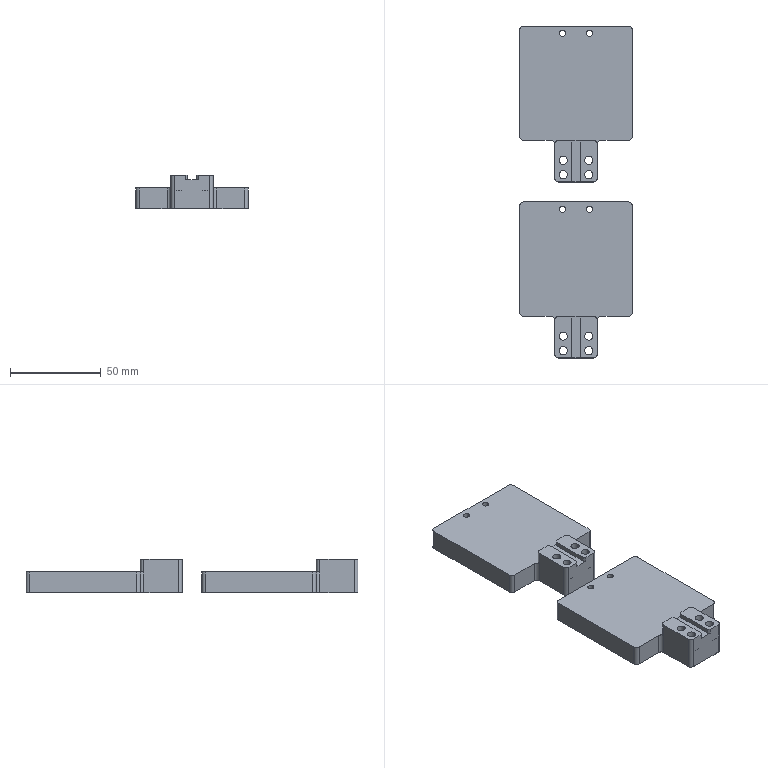NC program | NX | posted with a generic post | part box 62 x 183 x 18.5 mm
Whole program:
N10 G17 G21 G94 G90
(FLOOR_WALL_COPY , TOOL : D80)
N12 T19 M6
N14 G54
N16 G17 G0 G90 X226. Y31. S6500 M3
N18 G43 Z30. H19
N20 Z9.
N22 G94 G1 Z6. F1500.
N24 X223.
N26 X-40.
N28 X-43.
N30 Z9.
N32 G0 Z30.
N34 X226.
N36 Z8.
N38 G1 Z5.
N40 X223.
N42 X-40.
N44 X-43.
N46 Z8.
N48 G0 Z30.
N50 X226.
N52 Z7.
N54 G1 Z4.
N56 X223.
N58 X-40.
N60 X-43.
N62 Z7.
N64 G0 Z30.
N66 X226.
N68 Z6.
N70 G1 Z3.
N72 X223.
N74 X-40.
N76 X-43.
N78 Z6.
N80 G0 Z30.
N82 X226.
N84 Z5.
N86 G1 Z2.
N88 X223.
N90 X-40.
N92 X-43.
N94 Z5.
N96 G0 Z30.
N98 X226.
N100 Z4.
N102 G1 Z1.
N104 X223.
N106 X-40.
N108 X-43.
N110 Z4.
N112 G0 Z30.
N114 X226.
N116 Z3.
N118 G1 Z0.
N120 X223.
N122 X-40.
N124 X-43.
N126 Z3.
N128 G0 Z30.
N130 M5
(FLOOR_WALL_1 , TOOL : D10)
N132 T15 M6
N134 G54
N136 G17 G0 G90 X-6.5 Y26.67 S9500 M3
N138 G43 Z30. H15
N140 Z0.514
N142 G94 G1 Z-0.986 F1000.
N144 X-0.5 Y30.134
N146 G3 X0. Y31. R1.
N148 G1 Y60. F3500.
N150 G2 X2. Y62. R2.
N152 G1 X61.
N154 G2 X63. Y60. R2.
N156 G1 Y47.512
N158 G3 X57.9 Y40.7 R7.1
N160 G1 Y21.3
N162 G3 X63. Y14.488 R7.1
N164 G1 Y2.
N166 G2 X61. Y0. R2.
N168 G1 X2.
N170 G2 X0. Y2. R2.
N172 G1 Y31.
N174 X5.
N176 Y57.
N178 X58.
N180 Y50.57
N182 G3 X52.9 Y40.7 R12.1
N184 G1 Y21.3
N186 G3 X58. Y11.43 R12.1
N188 G1 Y5.
N190 X5.
N192 Y31.
N194 X10.
N196 Y52.
N198 X52.166
N200 G3 X47.9 Y40.7 R17.1
N202 G1 Y21.3
N204 G3 X52.166 Y10. R17.1
N206 G1 X10.
N208 Y31.
N210 X15.
N212 Y47.
N214 X43.817
N216 G3 X42.9 Y40.7 R22.1
N218 G1 Y21.3
N220 G3 X43.817 Y15. R22.1
N222 G1 X15.
N224 Y31.
N226 X20.
N228 Y42.
N230 X37.931
N232 G3 X37.9 Y40.7 R27.1
N234 G1 Y21.3
N236 G3 X37.931 Y20. R27.1
N238 G1 X20.
N240 Y31.
N242 X25.
N244 Y37.
N246 X32.9
N248 Y25.
N250 X25.
N252 Y31.
N254 G3 X24.5 Y31.866 R1.
N256 G1 Z0.514
N258 G0 X-6.5 Y26.67 Z-0.471
N260 G1 Z-1.971 F1000.
N262 X-0.5 Y30.134
N264 G3 X0. Y31. R1.
N266 G1 Y60. F3500.
N268 G2 X2. Y62. R2.
N270 G1 X61.
N272 G2 X63. Y60. R2.
N274 G1 Y47.512
N276 G3 X57.9 Y40.7 R7.1
N278 G1 Y21.3
N280 G3 X63. Y14.488 R7.1
N282 G1 Y2.
N284 G2 X61. Y0. R2.
N286 G1 X2.
N288 G2 X0. Y2. R2.
N290 G1 Y31.
N292 X5.
N294 Y57.
N296 X58.
N298 Y50.57
N300 G3 X52.9 Y40.7 R12.1
N302 G1 Y21.3
N304 G3 X58. Y11.43 R12.1
N306 G1 Y5.
N308 X5.
N310 Y31.
N312 X10.
N314 Y52.
N316 X52.166
N318 G3 X47.9 Y40.7 R17.1
N320 G1 Y21.3
N322 G3 X52.166 Y10. R17.1
N324 G1 X10.
N326 Y31.
N328 X15.
N330 Y47.
N332 X43.817
N334 G3 X42.9 Y40.7 R22.1
N336 G1 Y21.3
N338 G3 X43.817 Y15. R22.1
N340 G1 X15.
N342 Y31.
N344 X20.
N346 Y42.
N348 X37.931
N350 G3 X37.9 Y40.7 R27.1
N352 G1 Y21.3
N354 G3 X37.931 Y20. R27.1
N356 G1 X20.
N358 Y31.
N360 X25.
N362 Y37.
N364 X32.9
N366 Y25.
N368 X25.
N370 Y31.
N372 G3 X24.5 Y31.866 R1.
N374 G1 Z-0.471
N376 G0 X-6.5 Y26.67 Z-1.457
N378 G1 Z-2.957 F1000.
N380 X-0.5 Y30.134
N382 G3 X0. Y31. R1.
N384 G1 Y60. F3500.
N386 G2 X2. Y62. R2.
N388 G1 X61.
N390 G2 X63. Y60. R2.
N392 G1 Y47.512
N394 G3 X57.9 Y40.7 R7.1
N396 G1 Y21.3
N398 G3 X63. Y14.488 R7.1
N400 G1 Y2.
N402 G2 X61. Y0. R2.
N404 G1 X2.
N406 G2 X0. Y2. R2.
N408 G1 Y31.
N410 X5.
N412 Y57.
N414 X58.
N416 Y50.57
N418 G3 X52.9 Y40.7 R12.1
N420 G1 Y21.3
N422 G3 X58. Y11.43 R12.1
N424 G1 Y5.
N426 X5.
N428 Y31.
N430 X10.
N432 Y52.
N434 X52.166
N436 G3 X47.9 Y40.7 R17.1
N438 G1 Y21.3
N440 G3 X52.166 Y10. R17.1
N442 G1 X10.
N444 Y31.
N446 X15.
N448 Y47.
N450 X43.817
N452 G3 X42.9 Y40.7 R22.1
N454 G1 Y21.3
N456 G3 X43.817 Y15. R22.1
N458 G1 X15.
N460 Y31.
N462 X20.
N464 Y42.
N466 X37.931
N468 G3 X37.9 Y40.7 R27.1
N470 G1 Y21.3
N472 G3 X37.931 Y20. R27.1
N474 G1 X20.
N476 Y31.
N478 X25.
N480 Y37.
N482 X32.9
N484 Y25.
N486 X25.
N488 Y31.
N490 G3 X24.5 Y31.866 R1.
N492 G1 Z-1.457
N494 G0 X-6.5 Y26.67 Z-2.443
N496 G1 Z-3.943 F1000.
N498 X-0.5 Y30.134
N500 G3 X0. Y31. R1.
N502 G1 Y60. F3500.
N504 G2 X2. Y62. R2.
N506 G1 X61.
N508 G2 X63. Y60. R2.
N510 G1 Y47.512
N512 G3 X57.9 Y40.7 R7.1
N514 G1 Y21.3
N516 G3 X63. Y14.488 R7.1
N518 G1 Y2.
N520 G2 X61. Y0. R2.
N522 G1 X2.
N524 G2 X0. Y2. R2.
N526 G1 Y31.
N528 X5.
N530 Y57.
N532 X58.
N534 Y50.57
N536 G3 X52.9 Y40.7 R12.1
N538 G1 Y21.3
N540 G3 X58. Y11.43 R12.1
N542 G1 Y5.
N544 X5.
N546 Y31.
N548 X10.
N550 Y52.
N552 X52.166
N554 G3 X47.9 Y40.7 R17.1
N556 G1 Y21.3
N558 G3 X52.166 Y10. R17.1
N560 G1 X10.
N562 Y31.
N564 X15.
N566 Y47.
N568 X43.817
N570 G3 X42.9 Y40.7 R22.1
N572 G1 Y21.3
N574 G3 X43.817 Y15. R22.1
N576 G1 X15.
N578 Y31.
N580 X20.
N582 Y42.
N584 X37.931
N586 G3 X37.9 Y40.7 R27.1
N588 G1 Y21.3
N590 G3 X37.931 Y20. R27.1
N592 G1 X20.
N594 Y31.
N596 X25.
N598 Y37.
N600 X32.9
N602 Y25.
N604 X25.
N606 Y31.
N608 G3 X24.5 Y31.866 R1.
N610 G1 Z-2.443
N612 G0 X-6.5 Y26.67 Z-3.429
N614 G1 Z-4.929 F1000.
N616 X-0.5 Y30.134
N618 G3 X0. Y31. R1.
N620 G1 Y60. F3500.
N622 G2 X2. Y62. R2.
N624 G1 X61.
N626 G2 X63. Y60. R2.
N628 G1 Y47.512
N630 G3 X57.9 Y40.7 R7.1
N632 G1 Y21.3
N634 G3 X63. Y14.488 R7.1
N636 G1 Y2.
N638 G2 X61. Y0. R2.
N640 G1 X2.
N642 G2 X0. Y2. R2.
N644 G1 Y31.
N646 X5.
N648 Y57.
N650 X58.
N652 Y50.57
N654 G3 X52.9 Y40.7 R12.1
N656 G1 Y21.3
N658 G3 X58. Y11.43 R12.1
N660 G1 Y5.
N662 X5.
N664 Y31.
N666 X10.
N668 Y52.
N670 X52.166
N672 G3 X47.9 Y40.7 R17.1
N674 G1 Y21.3
N676 G3 X52.166 Y10. R17.1
N678 G1 X10.
N680 Y31.
N682 X15.
N684 Y47.
N686 X43.817
N688 G3 X42.9 Y40.7 R22.1
N690 G1 Y21.3
N692 G3 X43.817 Y15. R22.1
N694 G1 X15.
N696 Y31.
N698 X20.
N700 Y42.
N702 X37.931
N704 G3 X37.9 Y40.7 R27.1
N706 G1 Y21.3
N708 G3 X37.931 Y20. R27.1
N710 G1 X20.
N712 Y31.
N714 X25.
N716 Y37.
N718 X32.9
N720 Y25.
N722 X25.
N724 Y31.
N726 G3 X24.5 Y31.866 R1.
N728 G1 Z-3.429
N730 G0 X-6.5 Y26.67 Z-4.414
N732 G1 Z-5.914 F1000.
N734 X-0.5 Y30.134
N736 G3 X0. Y31. R1.
N738 G1 Y60. F3500.
N740 G2 X2. Y62. R2.
N742 G1 X61.
N744 G2 X63. Y60. R2.
N746 G1 Y47.512
N748 G3 X57.9 Y40.7 R7.1
N750 G1 Y21.3
N752 G3 X63. Y14.488 R7.1
N754 G1 Y2.
N756 G2 X61. Y0. R2.
N758 G1 X2.
N760 G2 X0. Y2. R2.
N762 G1 Y31.
N764 X5.
N766 Y57.
N768 X58.
N770 Y50.57
N772 G3 X52.9 Y40.7 R12.1
N774 G1 Y21.3
N776 G3 X58. Y11.43 R12.1
N778 G1 Y5.
N780 X5.
N782 Y31.
N784 X10.
N786 Y52.
N788 X52.166
N790 G3 X47.9 Y40.7 R17.1
N792 G1 Y21.3
N794 G3 X52.166 Y10. R17.1
N796 G1 X10.
N798 Y31.
N800 X15.
N802 Y47.
N804 X43.817
N806 G3 X42.9 Y40.7 R22.1
N808 G1 Y21.3
N810 G3 X43.817 Y15. R22.1
N812 G1 X15.
N814 Y31.
N816 X20.
N818 Y42.
N820 X37.931
N822 G3 X37.9 Y40.7 R27.1
N824 G1 Y21.3
N826 G3 X37.931 Y20. R27.1
N828 G1 X20.
N830 Y31.
N832 X25.
N834 Y37.
N836 X32.9
N838 Y25.
N840 X25.
N842 Y31.
N844 G3 X24.5 Y31.866 R1.
N846 G1 Z-4.414
N848 G0 X-6.5 Y26.67 Z-5.4
N850 G1 Z-6.9 F1000.
N852 X-0.5 Y30.134
N854 G3 X0. Y31. R1.
N856 G1 Y60. F3500.
N858 G2 X2. Y62. R2.
N860 G1 X61.
N862 G2 X63. Y60. R2.
N864 G1 Y47.512
N866 G3 X57.9 Y40.7 R7.1
N868 G1 Y21.3
N870 G3 X63. Y14.488 R7.1
N872 G1 Y2.
N874 G2 X61. Y0. R2.
N876 G1 X2.
N878 G2 X0. Y2. R2.
N880 G1 Y31.
N882 X5.
N884 Y57.
N886 X58.
N888 Y50.57
N890 G3 X52.9 Y40.7 R12.1
N892 G1 Y21.3
N894 G3 X58. Y11.43 R12.1
N896 G1 Y5.
N898 X5.
N900 Y31.
N902 X10.
N904 Y52.
N906 X52.166
N908 G3 X47.9 Y40.7 R17.1
N910 G1 Y21.3
N912 G3 X52.166 Y10. R17.1
N914 G1 X10.
N916 Y31.
N918 X15.
N920 Y47.
N922 X43.817
N924 G3 X42.9 Y40.7 R22.1
N926 G1 Y21.3
N928 G3 X43.817 Y15. R22.1
N930 G1 X15.
N932 Y31.
N934 X20.
N936 Y42.
N938 X37.931
N940 G3 X37.9 Y40.7 R27.1
N942 G1 Y21.3
N944 G3 X37.931 Y20. R27.1
N946 G1 X20.
N948 Y31.
N950 X25.
N952 Y37.
N954 X32.9
N956 Y25.
N958 X25.
N960 Y31.
N962 G3 X24.5 Y31.866 R1.
N964 G1 Z-5.4
N966 G0 Z30.
N968 X130.28 Y-6.5
N970 Z0.514
N972 G1 Z-0.986 F1000.
N974 X126.816 Y-0.5
N976 G3 X125.95 Y0. R1.
N978 G1 X99. F3500.
N980 G2 X97. Y2. R2.
N982 G1 Y60.
N984 G2 X99. Y62. R2.
N986 G1 X158.
N988 G2 X160. Y60. R2.
N990 G1 Y47.512
N992 G3 X154.9 Y40.7 R7.1
N994 G1 Y21.3
N996 G3 X160. Y14.488 R7.1
N998 G1 Y2.
N1000 G2 X158. Y0. R2.
N1002 G1 X125.95
N1004 Y5.
N1006 X102.
N1008 Y57.
N1010 X155.
N1012 Y50.57
N1014 G3 X149.9 Y40.7 R12.1
N1016 G1 Y21.3
N1018 G3 X155. Y11.43 R12.1
N1020 G1 Y5.
N1022 X125.95
N1024 Y10.
N1026 X107.
N1028 Y52.
N1030 X149.166
N1032 G3 X144.9 Y40.7 R17.1
N1034 G1 Y21.3
N1036 G3 X149.166 Y10. R17.1
N1038 G1 X125.95
N1040 Y15.
N1042 X112.
N1044 Y47.
N1046 X140.817
N1048 G3 X139.9 Y40.7 R22.1
N1050 G1 Y21.3
N1052 G3 X140.817 Y15. R22.1
N1054 G1 X125.95
N1056 Y20.
N1058 X117.
N1060 Y42.
N1062 X134.931
N1064 G3 X134.9 Y40.7 R27.1
N1066 G1 Y21.3
N1068 G3 X134.931 Y20. R27.1
N1070 G1 X125.95
N1072 Y25.
N1074 X122.
N1076 Y37.
N1078 X129.9
N1080 Y25.
N1082 X125.95
N1084 G3 X125.084 Y24.5 R1.
N1086 G1 Z0.514
N1088 G0 X130.28 Y-6.5 Z-0.471
N1090 G1 Z-1.971 F1000.
N1092 X126.816 Y-0.5
N1094 G3 X125.95 Y0. R1.
N1096 G1 X99. F3500.
N1098 G2 X97. Y2. R2.
N1100 G1 Y60.
N1102 G2 X99. Y62. R2.
N1104 G1 X158.
N1106 G2 X160. Y60. R2.
N1108 G1 Y47.512
N1110 G3 X154.9 Y40.7 R7.1
N1112 G1 Y21.3
N1114 G3 X160. Y14.488 R7.1
N1116 G1 Y2.
N1118 G2 X158. Y0. R2.
N1120 G1 X125.95
N1122 Y5.
N1124 X102.
N1126 Y57.
N1128 X155.
N1130 Y50.57
N1132 G3 X149.9 Y40.7 R12.1
N1134 G1 Y21.3
N1136 G3 X155. Y11.43 R12.1
N1138 G1 Y5.
N1140 X125.95
N1142 Y10.
N1144 X107.
N1146 Y52.
N1148 X149.166
N1150 G3 X144.9 Y40.7 R17.1
N1152 G1 Y21.3
N1154 G3 X149.166 Y10. R17.1
N1156 G1 X125.95
N1158 Y15.
N1160 X112.
N1162 Y47.
N1164 X140.817
N1166 G3 X139.9 Y40.7 R22.1
N1168 G1 Y21.3
N1170 G3 X140.817 Y15. R22.1
N1172 G1 X125.95
N1174 Y20.
N1176 X117.
N1178 Y42.
N1180 X134.931
N1182 G3 X134.9 Y40.7 R27.1
N1184 G1 Y21.3
N1186 G3 X134.931 Y20. R27.1
N1188 G1 X125.95
N1190 Y25.
N1192 X122.
N1194 Y37.
N1196 X129.9
N1198 Y25.
N1200 X125.95
N1202 G3 X125.084 Y24.5 R1.
N1204 G1 Z-0.471
N1206 G0 X130.28 Y-6.5 Z-1.457
N1208 G1 Z-2.957 F1000.
N1210 X126.816 Y-0.5
N1212 G3 X125.95 Y0. R1.
N1214 G1 X99. F3500.
N1216 G2 X97. Y2. R2.
N1218 G1 Y60.
N1220 G2 X99. Y62. R2.
N1222 G1 X158.
N1224 G2 X160. Y60. R2.
N1226 G1 Y47.512
N1228 G3 X154.9 Y40.7 R7.1
N1230 G1 Y21.3
N1232 G3 X160. Y14.488 R7.1
N1234 G1 Y2.
N1236 G2 X158. Y0. R2.
N1238 G1 X125.95
N1240 Y5.
N1242 X102.
N1244 Y57.
N1246 X155.
N1248 Y50.57
N1250 G3 X149.9 Y40.7 R12.1
N1252 G1 Y21.3
N1254 G3 X155. Y11.43 R12.1
N1256 G1 Y5.
N1258 X125.95
N1260 Y10.
N1262 X107.
N1264 Y52.
N1266 X149.166
N1268 G3 X144.9 Y40.7 R17.1
N1270 G1 Y21.3
N1272 G3 X149.166 Y10. R17.1
N1274 G1 X125.95
N1276 Y15.
N1278 X112.
N1280 Y47.
N1282 X140.817
N1284 G3 X139.9 Y40.7 R22.1
N1286 G1 Y21.3
N1288 G3 X140.817 Y15. R22.1
N1290 G1 X125.95
N1292 Y20.
N1294 X117.
N1296 Y42.
N1298 X134.931
N1300 G3 X134.9 Y40.7 R27.1
N1302 G1 Y21.3
N1304 G3 X134.931 Y20. R27.1
N1306 G1 X125.95
N1308 Y25.
N1310 X122.
N1312 Y37.
N1314 X129.9
N1316 Y25.
N1318 X125.95
N1320 G3 X125.084 Y24.5 R1.
N1322 G1 Z-1.457
N1324 G0 X130.28 Y-6.5 Z-2.443
N1326 G1 Z-3.943 F1000.
N1328 X126.816 Y-0.5
N1330 G3 X125.95 Y0. R1.
N1332 G1 X99. F3500.
N1334 G2 X97. Y2. R2.
N1336 G1 Y60.
N1338 G2 X99. Y62. R2.
N1340 G1 X158.
N1342 G2 X160. Y60. R2.
N1344 G1 Y47.512
N1346 G3 X154.9 Y40.7 R7.1
N1348 G1 Y21.3
N1350 G3 X160. Y14.488 R7.1
N1352 G1 Y2.
N1354 G2 X158. Y0. R2.
N1356 G1 X125.95
N1358 Y5.
N1360 X102.
N1362 Y57.
N1364 X155.
N1366 Y50.57
N1368 G3 X149.9 Y40.7 R12.1
N1370 G1 Y21.3
N1372 G3 X155. Y11.43 R12.1
N1374 G1 Y5.
N1376 X125.95
N1378 Y10.
N1380 X107.
N1382 Y52.
N1384 X149.166
N1386 G3 X144.9 Y40.7 R17.1
N1388 G1 Y21.3
N1390 G3 X149.166 Y10. R17.1
N1392 G1 X125.95
N1394 Y15.
N1396 X112.
N1398 Y47.
N1400 X140.817
N1402 G3 X139.9 Y40.7 R22.1
N1404 G1 Y21.3
N1406 G3 X140.817 Y15. R22.1
N1408 G1 X125.95
N1410 Y20.
N1412 X117.
N1414 Y42.
N1416 X134.931
N1418 G3 X134.9 Y40.7 R27.1
N1420 G1 Y21.3
N1422 G3 X134.931 Y20. R27.1
N1424 G1 X125.95
N1426 Y25.
N1428 X122.
N1430 Y37.
N1432 X129.9
N1434 Y25.
N1436 X125.95
N1438 G3 X125.084 Y24.5 R1.
N1440 G1 Z-2.443
N1442 G0 X130.28 Y-6.5 Z-3.429
N1444 G1 Z-4.929 F1000.
N1446 X126.816 Y-0.5
N1448 G3 X125.95 Y0. R1.
N1450 G1 X99. F3500.
N1452 G2 X97. Y2. R2.
N1454 G1 Y60.
N1456 G2 X99. Y62. R2.
N1458 G1 X158.
N1460 G2 X160. Y60. R2.
N1462 G1 Y47.512
N1464 G3 X154.9 Y40.7 R7.1
N1466 G1 Y21.3
N1468 G3 X160. Y14.488 R7.1
N1470 G1 Y2.
N1472 G2 X158. Y0. R2.
N1474 G1 X125.95
N1476 Y5.
N1478 X102.
N1480 Y57.
N1482 X155.
N1484 Y50.57
N1486 G3 X149.9 Y40.7 R12.1
N1488 G1 Y21.3
N1490 G3 X155. Y11.43 R12.1
N1492 G1 Y5.
N1494 X125.95
N1496 Y10.
N1498 X107.
N1500 Y52.
N1502 X149.166
N1504 G3 X144.9 Y40.7 R17.1
N1506 G1 Y21.3
N1508 G3 X149.166 Y10. R17.1
N1510 G1 X125.95
N1512 Y15.
N1514 X112.
N1516 Y47.
N1518 X140.817
N1520 G3 X139.9 Y40.7 R22.1
N1522 G1 Y21.3
N1524 G3 X140.817 Y15. R22.1
N1526 G1 X125.95
N1528 Y20.
N1530 X117.
N1532 Y42.
N1534 X134.931
N1536 G3 X134.9 Y40.7 R27.1
N1538 G1 Y21.3
N1540 G3 X134.931 Y20. R27.1
N1542 G1 X125.95
N1544 Y25.
N1546 X122.
N1548 Y37.
N1550 X129.9
N1552 Y25.
N1554 X125.95
N1556 G3 X125.084 Y24.5 R1.
N1558 G1 Z-3.429
N1560 G0 X130.28 Y-6.5 Z-4.414
N1562 G1 Z-5.914 F1000.
N1564 X126.816 Y-0.5
N1566 G3 X125.95 Y0. R1.
N1568 G1 X99. F3500.
N1570 G2 X97. Y2. R2.
N1572 G1 Y60.
N1574 G2 X99. Y62. R2.
N1576 G1 X158.
N1578 G2 X160. Y60. R2.
N1580 G1 Y47.512
N1582 G3 X154.9 Y40.7 R7.1
N1584 G1 Y21.3
N1586 G3 X160. Y14.488 R7.1
N1588 G1 Y2.
N1590 G2 X158. Y0. R2.
N1592 G1 X125.95
N1594 Y5.
N1596 X102.
N1598 Y57.
N1600 X155.
N1602 Y50.57
N1604 G3 X149.9 Y40.7 R12.1
N1606 G1 Y21.3
N1608 G3 X155. Y11.43 R12.1
N1610 G1 Y5.
N1612 X125.95
N1614 Y10.
N1616 X107.
N1618 Y52.
N1620 X149.166
N1622 G3 X144.9 Y40.7 R17.1
N1624 G1 Y21.3
N1626 G3 X149.166 Y10. R17.1
N1628 G1 X125.95
N1630 Y15.
N1632 X112.
N1634 Y47.
N1636 X140.817
N1638 G3 X139.9 Y40.7 R22.1
N1640 G1 Y21.3
N1642 G3 X140.817 Y15. R22.1
N1644 G1 X125.95
N1646 Y20.
N1648 X117.
N1650 Y42.
N1652 X134.931
N1654 G3 X134.9 Y40.7 R27.1
N1656 G1 Y21.3
N1658 G3 X134.931 Y20. R27.1
N1660 G1 X125.95
N1662 Y25.
N1664 X122.
N1666 Y37.
N1668 X129.9
N1670 Y25.
N1672 X125.95
N1674 G3 X125.084 Y24.5 R1.
N1676 G1 Z-4.414
N1678 G0 X130.28 Y-6.5 Z-5.4
N1680 G1 Z-6.9 F1000.
N1682 X126.816 Y-0.5
N1684 G3 X125.95 Y0. R1.
N1686 G1 X99. F3500.
N1688 G2 X97. Y2. R2.
N1690 G1 Y60.
N1692 G2 X99. Y62. R2.
N1694 G1 X158.
N1696 G2 X160. Y60. R2.
N1698 G1 Y47.512
N1700 G3 X154.9 Y40.7 R7.1
N1702 G1 Y21.3
N1704 G3 X160. Y14.488 R7.1
N1706 G1 Y2.
N1708 G2 X158. Y0. R2.
N1710 G1 X125.95
N1712 Y5.
N1714 X102.
N1716 Y57.
N1718 X155.
N1720 Y50.57
N1722 G3 X149.9 Y40.7 R12.1
N1724 G1 Y21.3
N1726 G3 X155. Y11.43 R12.1
N1728 G1 Y5.
N1730 X125.95
N1732 Y10.
N1734 X107.
N1736 Y52.
N1738 X149.166
N1740 G3 X144.9 Y40.7 R17.1
N1742 G1 Y21.3
N1744 G3 X149.166 Y10. R17.1
N1746 G1 X125.95
N1748 Y15.
N1750 X112.
N1752 Y47.
N1754 X140.817
N1756 G3 X139.9 Y40.7 R22.1
N1758 G1 Y21.3
N1760 G3 X140.817 Y15. R22.1
N1762 G1 X125.95
N1764 Y20.
N1766 X117.
N1768 Y42.
N1770 X134.931
N1772 G3 X134.9 Y40.7 R27.1
N1774 G1 Y21.3
N1776 G3 X134.931 Y20. R27.1
N1778 G1 X125.95
N1780 Y25.
N1782 X122.
N1784 Y37.
N1786 X129.9
N1788 Y25.
N1790 X125.95
N1792 G3 X125.084 Y24.5 R1.
N1794 G1 Z-5.4
N1796 G0 Z30.
N1798 M5
(FLOOR_WALL_1_COPY , TOOL : D10JING)
N1800 T14 M6
N1802 G54
N1804 G17 G0 G90 X-1.091 Y-5.918 S9500 M3
N1806 G43 Z30. H14
N1808 Z-5.5
N1810 G94 G1 Z-7. F1000.
N1812 X-0.497 Y-5.575
N1814 G3 X0.003 Y-4.709 R1.
N1816 G1 Y66.709 F1500.
N1818 G2 X2. Y67. R7.
N1820 G1 X4.919
N1822 Y-5.
N1824 X9.836
N1826 Y67.
N1828 X14.752
N1830 Y-5.
N1832 X19.669
N1834 Y67.
N1836 X24.585
N1838 Y-5.
N1840 X29.501
N1842 Y67.
N1844 X34.418
N1846 Y-5.
N1848 X39.334
N1850 Y67.
N1852 X44.251
N1854 Y-5.
N1856 X49.167
N1858 Y67.
N1860 X54.084
N1862 Y-5.
N1864 X59.
N1866 Y16.8
N1868 G3 X58.796 Y16.96 R0.5
N1870 G1 Z-5.5
N1872 G0 X59. Y16.8
N1874 G1 Z-7. F1000.
N1876 G2 X57.5 Y21.3 R7.5
N1878 G1 Y40.7
N1880 G2 X59. Y45.2 R7.5
N1882 G1 Y67. F1500.
N1884 G3 X58.5 Y67.866 R1.
N1886 G1 X57.402 Y68.5
N1888 Z-5.5
N1890 G0 Z30.
N1892 X69.5 Y12.702
N1894 Z-5.5
N1896 G1 Z-7. F1000.
N1898 X68.866 Y13.8
N1900 G3 X68. Y14.3 R1.
N1902 G1 X65. F1500.
N1904 G2 X58. Y21.3 R7.
N1906 G1 Y40.7
N1908 G2 X65. Y47.7 R7.
N1910 G1 X68.
N1912 G3 X68.866 Y48.2 R1.
N1914 G1 X69.5 Y49.298
N1916 Z-5.5
N1918 G0 Z30.
N1920 X95.909 Y-5.918
N1922 Z-5.5
N1924 G1 Z-7. F1000.
N1926 X96.503 Y-5.575
N1928 G3 X97.003 Y-4.709 R1.
N1930 G1 Y66.709 F1500.
N1932 G2 X99. Y67. R7.
N1934 G1 X101.919
N1936 Y-5.
N1938 X106.836
N1940 Y67.
N1942 X111.752
N1944 Y-5.
N1946 X116.669
N1948 Y67.
N1950 X121.585
N1952 Y-5.
N1954 X126.501
N1956 Y67.
N1958 X131.418
N1960 Y-5.
N1962 X136.334
N1964 Y67.
N1966 X141.251
N1968 Y-5.
N1970 X146.167
N1972 Y67.
N1974 X151.084
N1976 Y-5.
N1978 X156.
N1980 Y16.8
N1982 G3 X155.796 Y16.96 R0.5
N1984 G1 Z-5.5
N1986 G0 X156. Y16.8
N1988 G1 Z-7. F1000.
N1990 G2 X154.5 Y21.3 R7.5
N1992 G1 Y40.7
N1994 G2 X156. Y45.2 R7.5
N1996 G1 Y67. F1500.
N1998 G3 X155.5 Y67.866 R1.
N2000 G1 X154.402 Y68.5
N2002 Z-5.5
N2004 G0 Z30.
N2006 X166.5 Y12.702
N2008 Z-5.5
N2010 G1 Z-7. F1000.
N2012 X165.866 Y13.8
N2014 G3 X165. Y14.3 R1.
N2016 G1 X162. F1500.
N2018 G2 X155. Y21.3 R7.
N2020 G1 Y40.7
N2022 G2 X162. Y47.7 R7.
N2024 G1 X165.
N2026 G3 X165.866 Y48.2 R1.
N2028 G1 X166.5 Y49.298
N2030 Z-5.5
N2032 G0 Z30.
N2034 M5
(FLOOR_WALL_1_COPY_1 , TOOL : D4)
N2036 T11 M6
N2038 G54
N2040 G17 G0 G90 X89.5 Y32.097 S9500 M3
N2042 G43 Z30. H11
N2044 Z1.1
N2046 G94 G1 Z-0.4 F1000.
N2048 X88.2 Y31.346
N2050 G3 X88. Y31. R0.4
N2052 G1 Y28.47 F2000.
N2054 X85.87 Y30.6
N2056 X63.13
N2058 X61.03 Y28.5
N2060 X61.
N2062 Y33.53
N2064 X63.13 Y31.4
N2066 X85.87
N2068 X88. Y33.53
N2070 Y31.
N2072 G3 X88.2 Y30.654 R0.4
N2074 G1 X89.5 Y29.903
N2076 Z1.1
N2078 G0 Y32.097 Z0.7
N2080 G1 Z-0.8 F1000.
N2082 X88.2 Y31.346
N2084 G3 X88. Y31. R0.4
N2086 G1 Y28.47 F2000.
N2088 X85.87 Y30.6
N2090 X63.13
N2092 X61.03 Y28.5
N2094 X61.
N2096 Y33.53
N2098 X63.13 Y31.4
N2100 X85.87
N2102 X88. Y33.53
N2104 Y31.
N2106 G3 X88.2 Y30.654 R0.4
N2108 G1 X89.5 Y29.903
N2110 Z0.7
N2112 G0 Y32.097 Z0.3
N2114 G1 Z-1.2 F1000.
N2116 X88.2 Y31.346
N2118 G3 X88. Y31. R0.4
N2120 G1 Y28.47 F2000.
N2122 X85.87 Y30.6
N2124 X63.13
N2126 X61.03 Y28.5
N2128 X61.
N2130 Y33.53
N2132 X63.13 Y31.4
N2134 X85.87
N2136 X88. Y33.53
N2138 Y31.
N2140 G3 X88.2 Y30.654 R0.4
N2142 G1 X89.5 Y29.903
N2144 Z0.3
N2146 G0 Y32.097 Z-0.1
N2148 G1 Z-1.6 F1000.
N2150 X88.2 Y31.346
N2152 G3 X88. Y31. R0.4
N2154 G1 Y28.47 F2000.
N2156 X85.87 Y30.6
N2158 X63.13
N2160 X61.03 Y28.5
N2162 X61.
N2164 Y33.53
N2166 X63.13 Y31.4
N2168 X85.87
N2170 X88. Y33.53
N2172 Y31.
N2174 G3 X88.2 Y30.654 R0.4
N2176 G1 X89.5 Y29.903
N2178 Z-0.1
N2180 G0 Y32.097 Z-0.5
N2182 G1 Z-2. F1000.
N2184 X88.2 Y31.346
N2186 G3 X88. Y31. R0.4
N2188 G1 Y28.47 F2000.
N2190 X85.87 Y30.6
N2192 X63.13
N2194 X61.03 Y28.5
N2196 X61.
N2198 Y33.53
N2200 X63.13 Y31.4
N2202 X85.87
N2204 X88. Y33.53
N2206 Y31.
N2208 G3 X88.2 Y30.654 R0.4
N2210 G1 X89.5 Y29.903
N2212 Z-0.5
N2214 G0 Y32.097 Z-0.9
N2216 G1 Z-2.4 F1000.
N2218 X88.2 Y31.346
N2220 G3 X88. Y31. R0.4
N2222 G1 Y28.47 F2000.
N2224 X85.87 Y30.6
N2226 X63.13
N2228 X61.03 Y28.5
N2230 X61.
N2232 Y33.53
N2234 X63.13 Y31.4
N2236 X85.87
N2238 X88. Y33.53
N2240 Y31.
N2242 G3 X88.2 Y30.654 R0.4
N2244 G1 X89.5 Y29.903
N2246 Z-0.9
N2248 G0 Z30.
N2250 X186.5 Y32.097
N2252 Z1.1
N2254 G1 Z-0.4 F1000.
N2256 X185.2 Y31.346
N2258 G3 X185. Y31. R0.4
N2260 G1 Y28.47 F2000.
N2262 X182.87 Y30.6
N2264 X160.13
N2266 X158.03 Y28.5
N2268 X158.
N2270 Y33.53
N2272 X160.13 Y31.4
N2274 X182.87
N2276 X185. Y33.53
N2278 Y31.
N2280 G3 X185.2 Y30.654 R0.4
N2282 G1 X186.5 Y29.903
N2284 Z1.1
N2286 G0 Y32.097 Z0.7
N2288 G1 Z-0.8 F1000.
N2290 X185.2 Y31.346
N2292 G3 X185. Y31. R0.4
N2294 G1 Y28.47 F2000.
N2296 X182.87 Y30.6
N2298 X160.13
N2300 X158.03 Y28.5
N2302 X158.
N2304 Y33.53
N2306 X160.13 Y31.4
N2308 X182.87
N2310 X185. Y33.53
N2312 Y31.
N2314 G3 X185.2 Y30.654 R0.4
N2316 G1 X186.5 Y29.903
N2318 Z0.7
N2320 G0 Y32.097 Z0.3
N2322 G1 Z-1.2 F1000.
N2324 X185.2 Y31.346
N2326 G3 X185. Y31. R0.4
N2328 G1 Y28.47 F2000.
N2330 X182.87 Y30.6
N2332 X160.13
N2334 X158.03 Y28.5
N2336 X158.
N2338 Y33.53
N2340 X160.13 Y31.4
N2342 X182.87
N2344 X185. Y33.53
N2346 Y31.
N2348 G3 X185.2 Y30.654 R0.4
N2350 G1 X186.5 Y29.903
N2352 Z0.3
N2354 G0 Y32.097 Z-0.1
N2356 G1 Z-1.6 F1000.
N2358 X185.2 Y31.346
N2360 G3 X185. Y31. R0.4
N2362 G1 Y28.47 F2000.
N2364 X182.87 Y30.6
N2366 X160.13
N2368 X158.03 Y28.5
N2370 X158.
N2372 Y33.53
N2374 X160.13 Y31.4
N2376 X182.87
N2378 X185. Y33.53
N2380 Y31.
N2382 G3 X185.2 Y30.654 R0.4
N2384 G1 X186.5 Y29.903
N2386 Z-0.1
N2388 G0 Y32.097 Z-0.5
N2390 G1 Z-2. F1000.
N2392 X185.2 Y31.346
N2394 G3 X185. Y31. R0.4
N2396 G1 Y28.47 F2000.
N2398 X182.87 Y30.6
N2400 X160.13
N2402 X158.03 Y28.5
N2404 X158.
N2406 Y33.53
N2408 X160.13 Y31.4
N2410 X182.87
N2412 X185. Y33.53
N2414 Y31.
N2416 G3 X185.2 Y30.654 R0.4
N2418 G1 X186.5 Y29.903
N2420 Z-0.5
N2422 G0 Y32.097 Z-0.9
N2424 G1 Z-2.4 F1000.
N2426 X185.2 Y31.346
N2428 G3 X185. Y31. R0.4
N2430 G1 Y28.47 F2000.
N2432 X182.87 Y30.6
N2434 X160.13
N2436 X158.03 Y28.5
N2438 X158.
N2440 Y33.53
N2442 X160.13 Y31.4
N2444 X182.87
N2446 X185. Y33.53
N2448 Y31.
N2450 G3 X185.2 Y30.654 R0.4
N2452 G1 X186.5 Y29.903
N2454 Z-0.9
N2456 G0 Z30.
(FLOOR_WALL_1_COPY_COPY , TOOL : D4)
N2458 X89.6 Y28.43
N2460 Z-1.
N2462 G1 Z-2.5 F1000.
N2464 X88.346 Y30.601
N2466 G3 X88. Y30.801 R0.4
N2468 G1 X61. F1500.
N2470 Y31.247
N2472 X63.001
N2474 X62.989 Y31.259
N2476 X62.554 Y31.694
N2478 X61.
N2480 Y32.14
N2482 X62.107
N2484 X61.661 Y32.586
N2486 X61.
N2488 G3 X60.654 Y32.386 R0.4
N2490 G1 X59.5 Y30.388
N2492 Z-1.
N2494 G0 X63.001 Y31.247
N2496 G1 Z-2.5 F1000.
N2498 X63.035 Y31.213
N2500 X63.081 Y31.196
N2502 X63.13 Y31.2
N2504 X85.87
N2506 X85.919 Y31.196
N2508 X85.965 Y31.213
N2510 X85.999 Y31.247
N2512 X88. F1500.
N2514 Y31.694
N2516 X86.446
N2518 X86.893 Y32.14
N2520 X88.
N2522 Y32.586
N2524 X87.339
N2526 G3 X87.235 Y32.2 R0.4
N2528 G1 X89.5
N2530 Z-1.
N2532 G0 X89.6 Y33.308
N2534 G1 Z-2.5 F1000.
N2536 X88.386 Y33.634
N2538 G3 X88. Y33.53 R0.4
N2540 G1 X85.87 Y31.4 F1500.
N2542 X63.13
N2544 X61.01 Y33.52
N2546 G3 X60.624 Y33.624 R0.4
N2548 G1 Y28.376
N2550 G3 X61.01 Y28.48 R0.4 F1000.
N2552 G1 X63.13 Y30.6 F1500.
N2554 X85.87
N2556 X88. Y28.47
N2558 G3 X88.386 Y28.366 R0.4
N2560 G1 X89.6 Y28.692
N2562 Z-1.
N2564 G0 Z30.
N2566 X186.6 Y28.43
N2568 Z-1.
N2570 G1 Z-2.5 F1000.
N2572 X185.346 Y30.601
N2574 G3 X185. Y30.801 R0.4
N2576 G1 X158. F1500.
N2578 Y31.247
N2580 X160.001
N2582 X159.989 Y31.259
N2584 X159.554 Y31.694
N2586 X158.
N2588 Y32.14
N2590 X159.107
N2592 X158.661 Y32.586
N2594 X158.
N2596 G3 X157.654 Y32.386 R0.4
N2598 G1 X156.5 Y30.388
N2600 Z-1.
N2602 G0 X160.001 Y31.247
N2604 G1 Z-2.5 F1000.
N2606 X160.035 Y31.213
N2608 X160.081 Y31.196
N2610 X160.13 Y31.2
N2612 X182.87
N2614 X182.919 Y31.196
N2616 X182.965 Y31.213
N2618 X182.999 Y31.247
N2620 X185. F1500.
N2622 Y31.694
N2624 X183.446
N2626 X183.893 Y32.14
N2628 X185.
N2630 Y32.586
N2632 X184.339
N2634 G3 X184.235 Y32.2 R0.4
N2636 G1 X186.5
N2638 Z-1.
N2640 G0 X186.6 Y33.308
N2642 G1 Z-2.5 F1000.
N2644 X185.386 Y33.634
N2646 G3 X185. Y33.53 R0.4
N2648 G1 X182.87 Y31.4 F1500.
N2650 X160.13
N2652 X158.01 Y33.52
N2654 G3 X157.624 Y33.624 R0.4
N2656 G1 Y28.376
N2658 G3 X158.01 Y28.48 R0.4 F1000.
N2660 G1 X160.13 Y30.6 F1500.
N2662 X182.87
N2664 X185. Y28.47
N2666 G3 X185.386 Y28.366 R0.4
N2668 G1 X186.6 Y28.692
N2670 Z-1.
N2672 G0 Z30.
N2674 M5
(PLANAR_MILL_COPY_COPY , TOOL : D6A45)
N2676 T01 M6
N2678 G54
N2680 G17 G0 G90 X81.134 Y23.05 S9500 M3
N2682 G43 Z30. H1
N2684 Z0.5
N2686 G94 G1 Z-1. F1250.
N2688 G3 X82. Y22.55 R1.
N2690 X83.35 Y23.9 R1.35
N2692 X82. Y22.55 R-1.35
N2694 X82.866 Y23.05 R1.
N2696 G1 Z0.5
N2698 G0 Z30.
N2700 X75.366 Y17.9
N2702 Z0.5
N2704 G1 Z-1.
N2706 G3 X74.5 Y18.4 R1.
N2708 G1 X65.
N2710 G2 X62.1 Y21.3 R2.9
N2712 G1 Y27.5
N2714 G2 X62.364 Y28.136 R0.9
N2716 G1 X63.364 Y29.136
N2718 G2 X64. Y29.4 R0.9
N2720 G1 X85.
N2722 G2 X85.636 Y29.136 R0.9
N2724 G1 X86.636 Y28.136
N2726 G2 X86.9 Y27.5 R0.9
N2728 G1 Y21.3
N2730 G2 X84. Y18.4 R2.9
N2732 G1 X74.5
N2734 G3 X73.634 Y17.9 R1.
N2736 G1 Z0.5
N2738 G0 Z30.
N2740 X73.134 Y23.05
N2742 Z0.5
N2744 G1 Z-1.
N2746 G3 X74. Y22.55 R1.
N2748 X75.35 Y23.9 R1.35
N2750 X74. Y22.55 R-1.35
N2752 X74.866 Y23.05 R1.
N2754 G1 Z0.5
N2756 G0 Z30.
N2758 Y38.95
N2760 Z0.5
N2762 G1 Z-1.
N2764 G3 X74. Y39.45 R1.
N2766 X72.65 Y38.1 R1.35
N2768 X74. Y39.45 R-1.35
N2770 X73.134 Y38.95 R1.
N2772 G1 Z0.5
N2774 G0 Z30.
N2776 X73.634 Y44.1
N2778 Z0.5
N2780 G1 Z-1.
N2782 G3 X74.5 Y43.6 R1.
N2784 G1 X84.
N2786 G2 X86.9 Y40.7 R2.9
N2788 G1 Y34.5
N2790 G2 X86.636 Y33.864 R0.9
N2792 G1 X85.636 Y32.864
N2794 G2 X85. Y32.6 R0.9
N2796 G1 X64.
N2798 G2 X63.364 Y32.864 R0.9
N2800 G1 X62.364 Y33.864
N2802 G2 X62.1 Y34.5 R0.9
N2804 G1 Y40.7
N2806 G2 X65. Y43.6 R2.9
N2808 G1 X74.5
N2810 G3 X75.366 Y44.1 R1.
N2812 G1 Z0.5
N2814 G0 Z30.
N2816 X82.866 Y38.95
N2818 Z0.5
N2820 G1 Z-1.
N2822 G3 X82. Y39.45 R1.
N2824 X80.65 Y38.1 R1.35
N2826 X82. Y39.45 R-1.35
N2828 X81.134 Y38.95 R1.
N2830 G1 Z0.5
N2832 G0 Z30.
N2834 X171.866
N2836 Z0.5
N2838 G1 Z-1.
N2840 G3 X171. Y39.45 R1.
N2842 X169.65 Y38.1 R1.35
N2844 X171. Y39.45 R-1.35
N2846 X170.134 Y38.95 R1.
N2848 G1 Z0.5
N2850 G0 Z30.
N2852 X170.634 Y44.1
N2854 Z0.5
N2856 G1 Z-1.
N2858 G3 X171.5 Y43.6 R1.
N2860 G1 X181.
N2862 G2 X183.9 Y40.7 R2.9
N2864 G1 Y34.5
N2866 G2 X183.636 Y33.864 R0.9
N2868 G1 X182.636 Y32.864
N2870 G2 X182. Y32.6 R0.9
N2872 G1 X161.
N2874 G2 X160.364 Y32.864 R0.9
N2876 G1 X159.364 Y33.864
N2878 G2 X159.1 Y34.5 R0.9
N2880 G1 Y40.7
N2882 G2 X162. Y43.6 R2.9
N2884 G1 X171.5
N2886 G3 X172.366 Y44.1 R1.
N2888 G1 Z0.5
N2890 G0 Z30.
N2892 X179.866 Y38.95
N2894 Z0.5
N2896 G1 Z-1.
N2898 G3 X179. Y39.45 R1.
N2900 X177.65 Y38.1 R1.35
N2902 X179. Y39.45 R-1.35
N2904 X178.134 Y38.95 R1.
N2906 G1 Z0.5
N2908 G0 Z30.
N2910 X179.85 Y23.034
N2912 Z0.5
N2914 G1 Z-1.
N2916 G3 X180.35 Y23.9 R1.
N2918 X179. Y25.25 R1.35
N2920 X180.35 Y23.9 R-1.35
N2922 X179.85 Y24.766 R1.
N2924 G1 Z0.5
N2926 G0 Z30.
N2928 X172.366 Y17.9
N2930 Z0.5
N2932 G1 Z-1.
N2934 G3 X171.5 Y18.4 R1.
N2936 G1 X162.
N2938 G2 X159.1 Y21.3 R2.9
N2940 G1 Y27.5
N2942 G2 X159.364 Y28.136 R0.9
N2944 G1 X160.364 Y29.136
N2946 G2 X161. Y29.4 R0.9
N2948 G1 X182.
N2950 G2 X182.636 Y29.136 R0.9
N2952 G1 X183.636 Y28.136
N2954 G2 X183.9 Y27.5 R0.9
N2956 G1 Y21.3
N2958 G2 X181. Y18.4 R2.9
N2960 G1 X171.5
N2962 G3 X170.634 Y17.9 R1.
N2964 G1 Z0.5
N2966 G0 Z30.
N2968 X170.134 Y23.05
N2970 Z0.5
N2972 G1 Z-1.
N2974 G3 X171. Y22.55 R1.
N2976 X172.35 Y23.9 R1.35
N2978 X171. Y22.55 R-1.35
N2980 X171.866 Y23.05 R1.
N2982 G1 Z0.5
N2984 G0 Z30.
(PLANAR_MILL_COPY_COPY_COPY , TOOL : D6A45)
N2986 X3.576 Y39.126
N2988 Z-6.5
N2990 G1 X3.448 Y39.052 Z-6.54
N2992 X3.25 Y38.714 Z-6.644
N2994 Y38.286 Z-6.759
N2996 X3.448 Y37.948 Z-6.864
N2998 X3.786 Y37.75 Z-6.969
N3000 X4.214 Z-7.084
N3002 X4.552 Y37.948 Z-7.189
N3004 X4.75 Y38.286 Z-7.294
N3006 Y38.714 Z-7.408
N3008 X4.552 Y39.052 Z-7.513
N3010 X4.214 Y39.25 Z-7.618
N3012 X3.786 Z-7.733
N3014 X3.448 Y39.052 Z-7.838
N3016 X3.25 Y38.714 Z-7.943
N3018 Y38.5 Z-8.
N3020 G3 X4. Y37.75 R0.75
N3022 X3.25 Y38.5 R-0.75
N3024 X3.5 Y38.067 R0.5
N3026 G1 Z-6.5
N3028 G0 Z30.
N3030 X3.576 Y24.126
N3032 Z-6.5
N3034 G1 X3.448 Y24.052 Z-6.54
N3036 X3.25 Y23.714 Z-6.644
N3038 Y23.286 Z-6.759
N3040 X3.448 Y22.948 Z-6.864
N3042 X3.786 Y22.75 Z-6.969
N3044 X4.214 Z-7.084
N3046 X4.552 Y22.948 Z-7.189
N3048 X4.75 Y23.286 Z-7.294
N3050 Y23.714 Z-7.408
N3052 X4.552 Y24.052 Z-7.513
N3054 X4.214 Y24.25 Z-7.618
N3056 X3.786 Z-7.733
N3058 X3.448 Y24.052 Z-7.838
N3060 X3.25 Y23.714 Z-7.943
N3062 Y23.5 Z-8.
N3064 G3 X4. Y22.75 R0.75
N3066 X3.25 Y23.5 R-0.75
N3068 X3.5 Y23.067 R0.5
N3070 G1 Z-6.5
N3072 G0 Z30.
N3074 X65.1 Y13.504
N3076 Z-6.5
N3078 G1 Z-8.
N3080 X64.66 Y14.751
N3082 G3 X63.9 Y15.402 R1.
N3084 G1 Y2.
N3086 G2 X61. Y-0.9 R2.9
N3088 G1 X2.
N3090 G2 X-0.9 Y2. R2.9
N3092 G1 Y60.
N3094 G2 X2. Y62.9 R2.9
N3096 G1 X61.
N3098 G2 X63.9 Y60. R2.9
N3100 G1 Y46.598
N3102 G3 X64.66 Y47.249 R1.
N3104 G1 X65.1 Y48.496
N3106 Z-6.5
N3108 G0 Z30.
N3110 X162.1 Y13.504
N3112 Z-6.5
N3114 G1 Z-8.
N3116 X161.66 Y14.751
N3118 G3 X160.9 Y15.402 R1.
N3120 G1 Y2.
N3122 G2 X158. Y-0.9 R2.9
N3124 G1 X99.
N3126 G2 X96.1 Y2. R2.9
N3128 G1 Y60.
N3130 G2 X99. Y62.9 R2.9
N3132 G1 X158.
N3134 G2 X160.9 Y60. R2.9
N3136 G1 Y46.598
N3138 G3 X161.66 Y47.249 R1.
N3140 G1 X162.1 Y48.496
N3142 Z-6.5
N3144 G0 Z30.
N3146 X100.374 Y23.076
N3148 Z-6.5
N3150 G1 X100.448 Y22.948 Z-6.54
N3152 X100.786 Y22.75 Z-6.644
N3154 X101.214 Z-6.759
N3156 X101.552 Y22.948 Z-6.864
N3158 X101.75 Y23.286 Z-6.969
N3160 Y23.714 Z-7.084
N3162 X101.552 Y24.052 Z-7.189
N3164 X101.214 Y24.25 Z-7.294
N3166 X100.786 Z-7.408
N3168 X100.448 Y24.052 Z-7.513
N3170 X100.25 Y23.714 Z-7.618
N3172 Y23.286 Z-7.733
N3174 X100.448 Y22.948 Z-7.838
N3176 X100.786 Y22.75 Z-7.943
N3178 X101. Z-8.
N3180 G3 X101.75 Y23.5 R0.75
N3182 X101. Y22.75 R-0.75
N3184 X101.433 Y23. R0.5
N3186 G1 Z-6.5
N3188 G0 Z30.
N3190 X101.626 Y38.924
N3192 Z-6.5
N3194 G1 X101.552 Y39.052 Z-6.54
N3196 X101.214 Y39.25 Z-6.644
N3198 X100.786 Z-6.759
N3200 X100.448 Y39.052 Z-6.864
N3202 X100.25 Y38.714 Z-6.969
N3204 Y38.286 Z-7.084
N3206 X100.448 Y37.948 Z-7.189
N3208 X100.786 Y37.75 Z-7.294
N3210 X101.214 Z-7.408
N3212 X101.552 Y37.948 Z-7.513
N3214 X101.75 Y38.286 Z-7.618
N3216 Y38.714 Z-7.733
N3218 X101.552 Y39.052 Z-7.838
N3220 X101.214 Y39.25 Z-7.943
N3222 X101. Z-8.
N3224 G3 X100.25 Y38.5 R0.75
N3226 X101. Y39.25 R-0.75
N3228 X100.567 Y39. R0.5
N3230 G1 Z-6.5
N3232 G0 Z30.
N3234 M5
(刀补4 , TOOL : D4)
N3236 T11 M6
N3238 G54
N3240 G17 G0 G90 X61.073 Y30.726 S9500 M3
N3242 G43 Z30. H11
N3244 Z-1.
N3246 G94 G1 Z-2.5 F1000.
N3248 G41 X61.164 Y30.684 D11
N3250 X62.614 Y30.296
N3252 G3 X63. Y30.399 R0.4
N3254 G1 X63.151 Y30.55 F1500.
N3256 X85.849
N3258 X86. Y30.399
N3260 G3 X86.386 Y30.296 R0.4
N3262 G40
N3264 G1 X86.477 Y30.338
N3266 Y31.662
N3268 G41 X86.386 Y31.704 F1000.
N3270 G3 X86. Y31.601 R0.4
N3272 G1 X85.849 Y31.45 F1500.
N3274 X63.151
N3276 X63. Y31.601
N3278 G3 X62.614 Y31.704 R0.4
N3280 G1 X61.164 Y31.316
N3282 G40
N3284 X61.073 Y31.274
N3286 Z-1.
N3288 G0 Z30.
N3290 X158.073 Y30.726
N3292 Z-1.
N3294 G1 Z-2.5 F1000.
N3296 G41 X158.164 Y30.684
N3298 X159.614 Y30.296
N3300 G3 X160. Y30.399 R0.4
N3302 G1 X160.151 Y30.55 F1500.
N3304 X182.849
N3306 X183. Y30.399
N3308 G3 X183.386 Y30.296 R0.4
N3310 G40
N3312 G1 X183.477 Y30.338
N3314 Y31.662
N3316 G41 X183.386 Y31.704 F1000.
N3318 G3 X183. Y31.601 R0.4
N3320 G1 X182.849 Y31.45 F1500.
N3322 X160.151
N3324 X160. Y31.601
N3326 G3 X159.614 Y31.704 R0.4
N3328 G1 X158.164 Y31.316
N3330 G40
N3332 X158.073 Y31.274
N3334 Z-1.
N3336 G0 Z30.
N3338 M5
N3340 M2